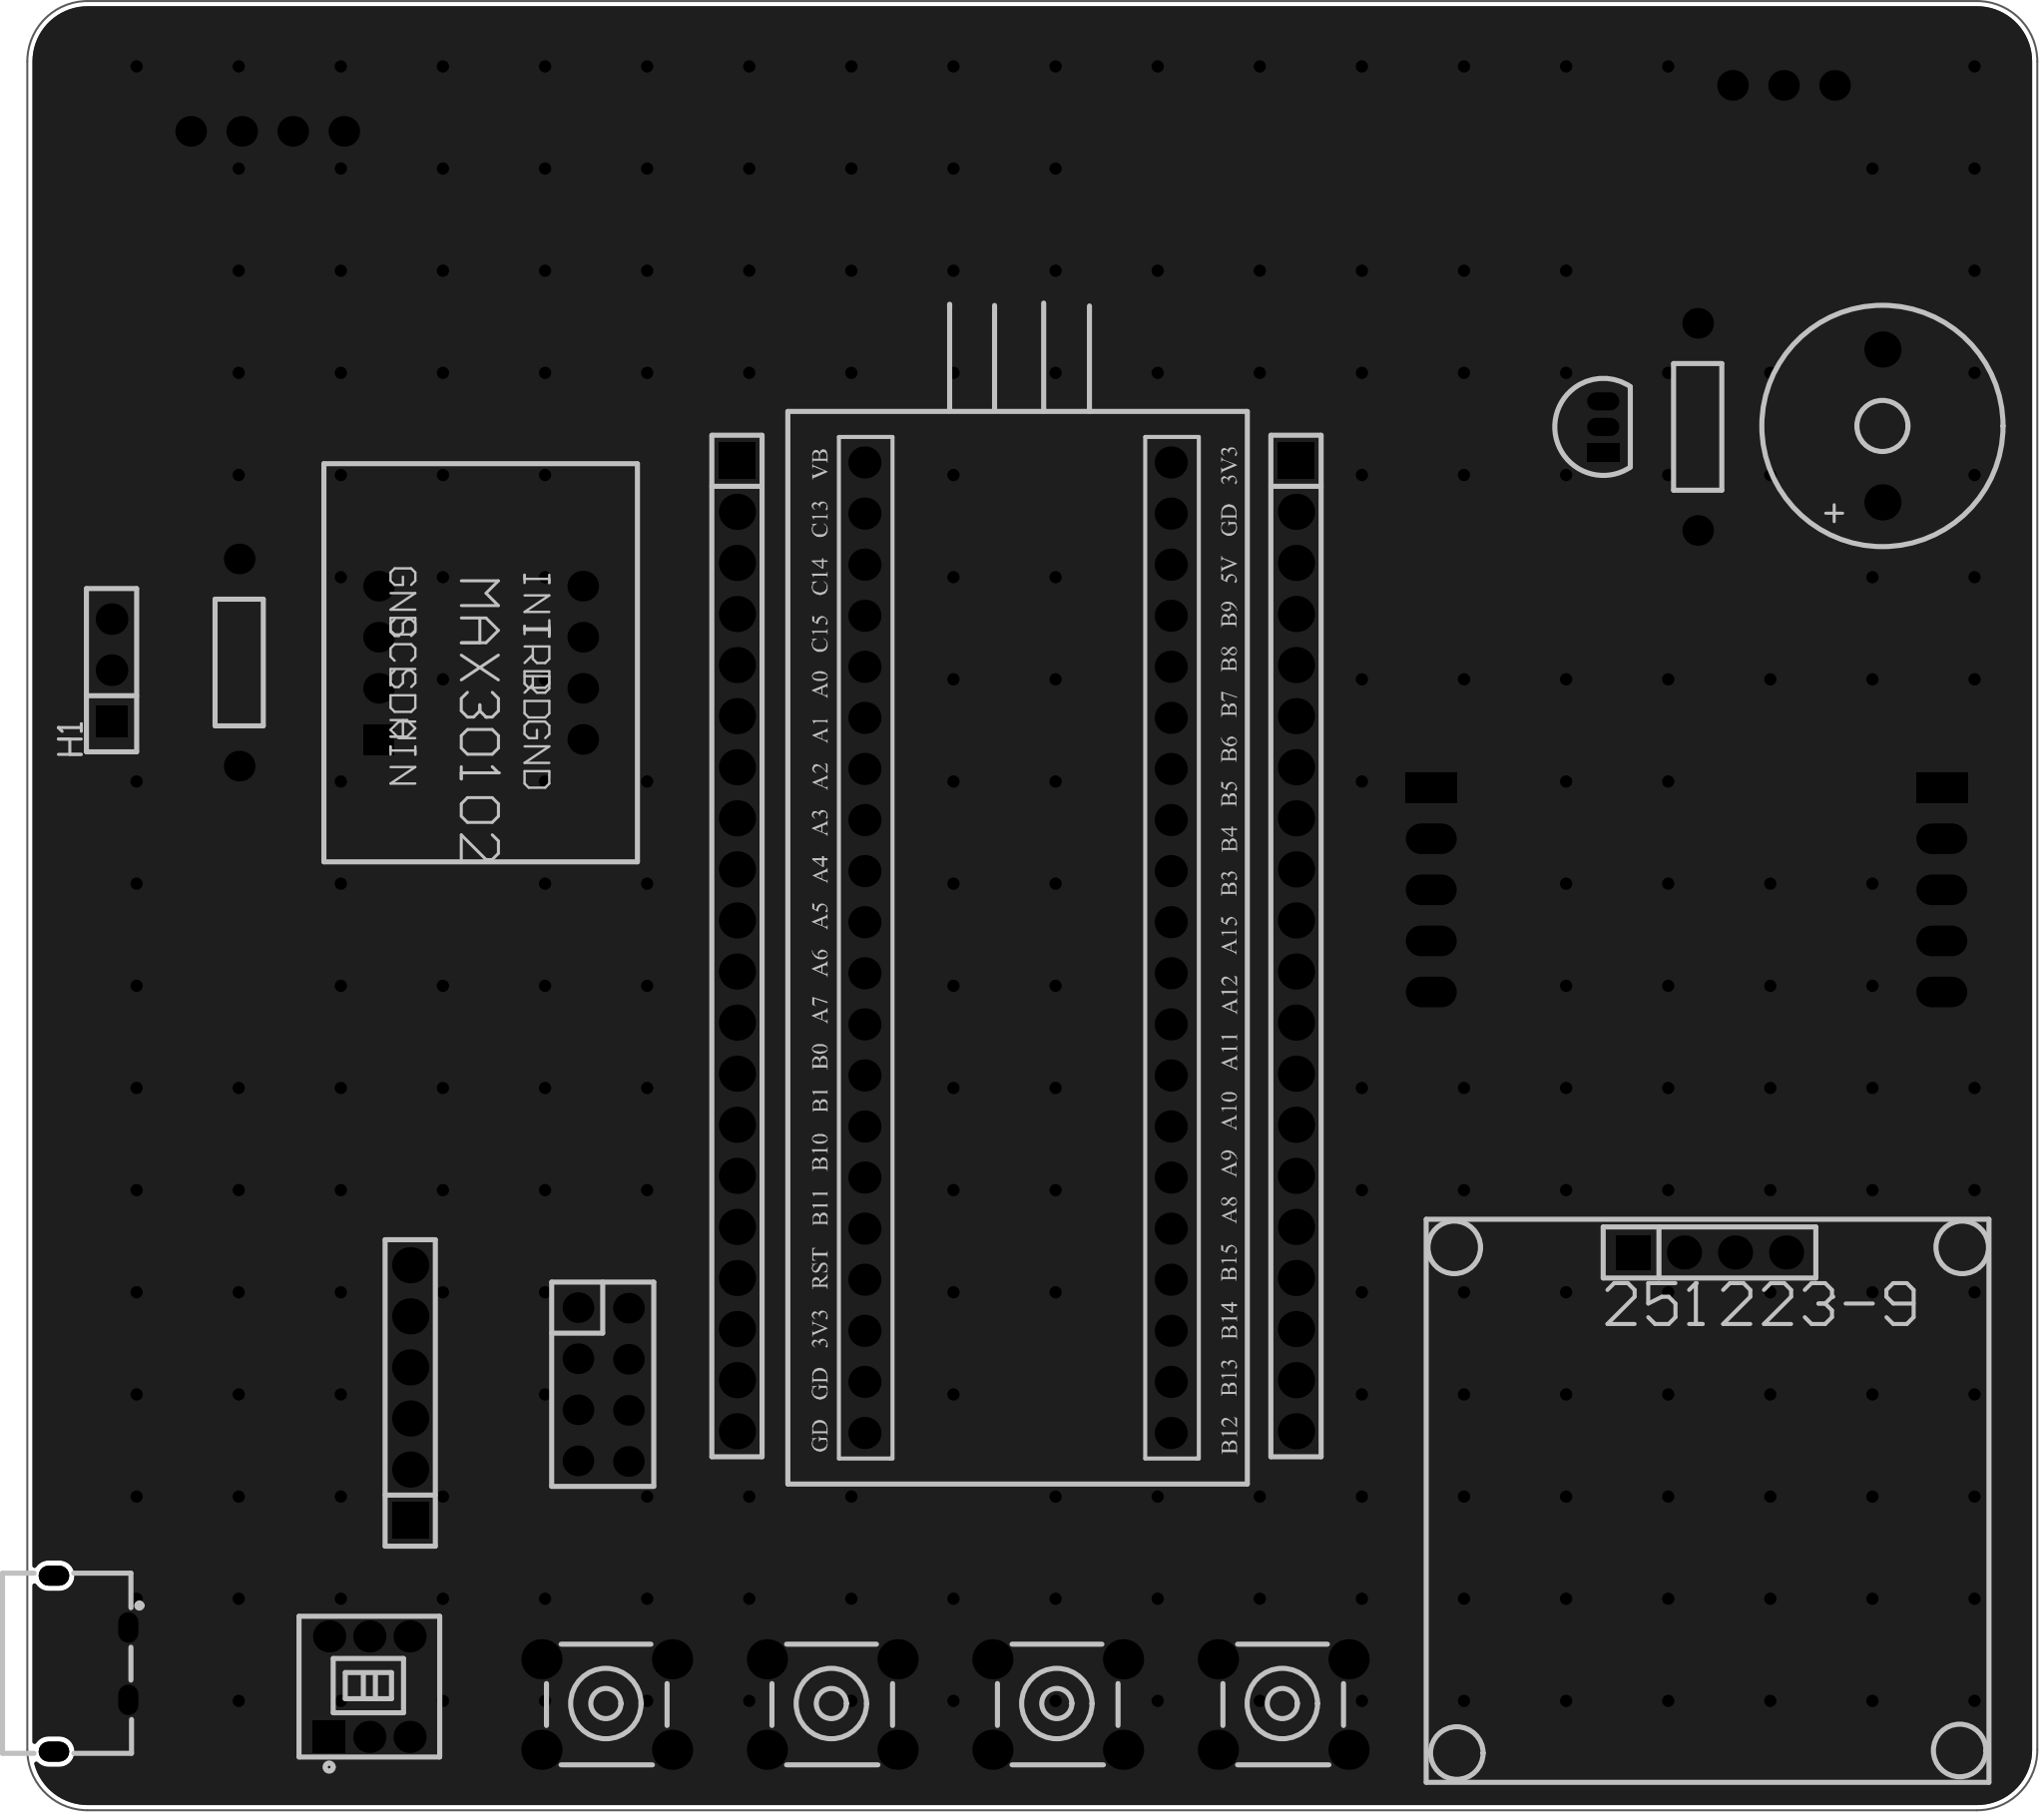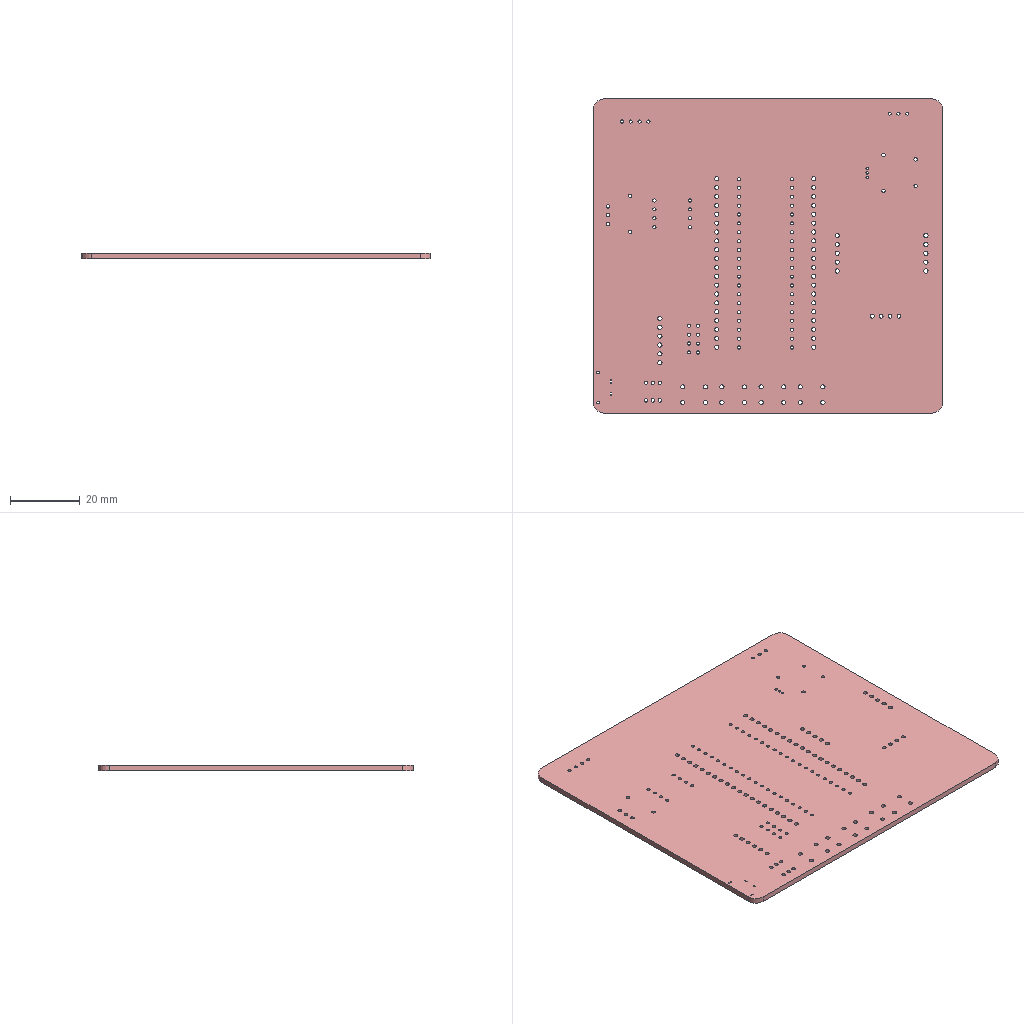Circuit board layout | Altium Designer | box 100 x 90 x 1.6 mm
Layer stack:
# Altium Designer layer stack of  (unit mm; dielectric type: 0 none, 1 core, 2 prepreg, 3 surface material)
index,name,kind,layer,copper_thickness_mm,dielectric_type,dielectric_thickness_mm,dielectric_material,dielectric_constant
0,Top Paste Mask Layer,other,,,,,,
1,Top Silkscreen Layer,other,,,,,,
2,Top Solder Mask Layer,dielectric,,,3,0.01,,3.3
3,Top Layer,copper,Top Layer,0.035,,,,
4,Dielectric1,dielectric,,,3,1.51,FR4,4.5
5,Bottom Layer,copper,Bottom Layer,0.035,,,,
6,Bottom Solder Mask Layer,dielectric,,,3,0.01,,3.3
7,Bottom Silkscreen Layer,other,,,,,,
8,Bottom Paste Mask Layer,other,,,,,,
# drill layer pairs: low layer,high layer
drill_pair,Top Layer,Bottom Layer
Part placement:
Designator,Comment,Layer,Footprint,Center-X(mm),Center-Y(mm),Rotation
H2,2.54-1*4P female,TopLayer,HDR-TH_4P-P2.54-V-F,165.672,135.255,0
H3,,TopLayer,HDR-TH_20P-P2.54-V-M-1,145.097,150.495,270
H4,,TopLayer,HDR-TH_20P-P2.54-V-M-1,117.284,150.495,270
H7,,TopLayer,HDR-TH_6P-P2.54-V-M-1,101.028,128.27,90
KEY1,Button 1,TopLayer,KEY-TH_4P-L6.0-W6.0-P4.50-LS7.5,110.808,112.776,0
KEY2,Button 5,TopLayer,KEY-TH_4P-L6.0-W6.0-P4.50-LS7.5,122.026,112.776,0
KEY3,Button 2,TopLayer,KEY-TH_4P-L6.0-W6.0-P4.50-LS7.5,133.244,112.776,0
KEY4,Button 4,TopLayer,KEY-TH_4P-L6.0-W6.0-P4.50-LS7.5,144.463,112.776,0
R98,4.7kΩ,TopLayer,Res_1/4W,92.519,164.592,90
U44,,TopLayer,STM32最小系统板,131.246,150.409,0
U89,,TopLayer,MAX30102,104.534,164.58,270
U98,,TopLayer,WiFi封装,110.629,128.688,90
SW8,TK-6700-1,TopLayer,SW-TH_TK-6700-1,98.996,113.665,0
U86,,TopLayer,ADXL345,164.529,153.289,0
USB2,KH-TYPE-C-2P,TopLayer,USB-SMD_KH-TYPE-C-2P,85.153,114.808,270
BUZZER3,2.3kHz,TopLayer,BUZ-TH_BD12.0-P7.60-D0.6-FD,174.274,176.356,90
Q17,,TopLayer,S8050_TO_92,160.384,176.31,90
R116,1kΩ,TopLayer,Res_1/4W,165.083,176.31,270
U1,,TopLayer,温湿度,169.355,193.294,180
U118,,TopLayer,MQ-X插件,93.916,191.008,90
H1,,TopLayer,HDR-TH_3P-P2.54-V-F,86.169,164.211,90
Pad and via stacks:
# Altium Designer via and pad stacks of  (unit mm). Each distinct definition once, with the count of objects using it.
# via: kind,start_layer,end_layer,hole_mm,diameter_mm,mode(0 simple;1 top-mid-bottom;2 full stack),diameter_per_layer,count,example_net
# pad: kind,layer,hole_mm,hole_type(0 round;1 square;2 slot),plating,top_size,top_shape(1 round;2 rect;3 octagon;9 rounded rect),mid_size,bottom_size,mode,footprint,size_per_layer,count,example
pad,Multi-Layer,1.1,0,plated,1.7x1.7,2,1.7x1.7,1.7x1.7,0,HDR-TH_4P-P2.54-V-F,,1,H2.1
pad,Multi-Layer,1.1,0,plated,1.7x1.7,1,1.7x1.7,1.7x1.7,0,HDR-TH_4P-P2.54-V-F,,3,H2.2
pad,Multi-Layer,1.2,0,plated,1.8x1.8,1,1.8x1.8,1.8x1.8,0,HDR-TH_20P-P2.54-V-M-1,,38,H3.20
pad,Multi-Layer,1.2,0,plated,1.8x1.8,2,1.8x1.8,1.8x1.8,0,HDR-TH_20P-P2.54-V-M-1,,2,H3.1
pad,Multi-Layer,1.2,0,plated,1.8x1.8,1,1.8x1.8,1.8x1.8,0,HDR-TH_6P-P2.54-V-M-1,,5,H7.6
pad,Multi-Layer,1.2,0,plated,1.8x1.8,2,1.8x1.8,1.8x1.8,0,HDR-TH_6P-P2.54-V-M-1,,1,H7.1
pad,Multi-Layer,1.2,0,plated,2x2,1,2x2,2x2,0,KEY-TH_4P-L6.0-W6.0-P4.50-LS7.5,,16,KEY1.1
pad,Multi-Layer,1,0,plated,1.524x1.524,1,1.524x1.524,1.524x1.524,0,Res_1/4W,,4,R98.1
pad,Multi-Layer,0.9,0,plated,1.6x1.6,1,1.6x1.6,1.6x1.6,0,STM32\u00D7\u00EE\u00D0\u00A1\u00CF\u00B5\u00CD\u00B3\u00B0\u00E5,,40,U44.40
pad,Multi-Layer,0.9144,0,plated,1.524x1.524,1,1.524x1.524,1.524x1.524,0,MAX30102,,7,U89.1
pad,Multi-Layer,0.9144,0,plated,1.524x1.524,2,1.524x1.524,1.524x1.524,0,MAX30102,,1,U89.8
pad,Multi-Layer,0.9144,0,plated,1.524x1.524,1,1.524x1.524,1.524x1.524,0,WiFi\u00B7\u00E2\u00D7\u00B0,,8,U98.1
pad,Multi-Layer,1,0,plated,1.6x1.6,2,1.6x1.6,1.6x1.6,0,SW-TH_TK-6700-1,,1,SW8.1
pad,Multi-Layer,1,0,plated,1.6x1.6,1,1.6x1.6,1.6x1.6,0,SW-TH_TK-6700-1,,5,SW8.2
pad,Multi-Layer,1.2,0,plated,1.524x2.54,1,1.524x2.54,1.524x2.54,0,ADXL345,,8,U86.5
pad,Multi-Layer,1.2,0,plated,1.524x2.54,2,1.524x2.54,1.524x2.54,0,ADXL345,,2,U86.1
pad,Multi-Layer,0.45,2,plated,1x1.524,1,1x1.524,1x1.524,0,USB-SMD_KH-TYPE-C-2P,,2,USB2.1
pad,Multi-Layer,0.5,2,plated,1x1.524,1,1x1.524,1x1.524,0,USB-SMD_KH-TYPE-C-2P,,2,USB2.3
pad,Multi-Layer,1,0,plated,1.8x1.8,1,1.8x1.8,1.8x1.8,0,BUZ-TH_BD12.0-P7.60-D0.6-FD,,2,BUZZER3.2
pad,Multi-Layer,0.701,0,plated,0.8992x1.6,2,0.8992x1.6,0.8992x1.6,0,S8050_TO_92,,1,Q17.1
pad,Multi-Layer,0.701,0,plated,0.8992x1.6,1,0.8992x1.6,0.8992x1.6,0,S8050_TO_92,,2,Q17.2
pad,Multi-Layer,0.9144,0,plated,1.524x1.524,1,1.524x1.524,1.524x1.524,0,\u00CE\u00C2\u00CA\u00AA\u00B6\u00C8,,3,U1.1
pad,Multi-Layer,0.9144,0,plated,1.524x1.524,1,1.524x1.524,1.524x1.524,0,MQ-X\u00B2\u00E5\u00BC\u00FE,,4,U118.1
pad,Multi-Layer,1.02,0,plated,1.575x1.575,1,1.575x1.575,1.575x1.575,0,HDR-TH_3P-P2.54-V-F,,2,H1.3
pad,Multi-Layer,1.02,0,plated,1.575x1.575,2,1.575x1.575,1.575x1.575,0,HDR-TH_3P-P2.54-V-F,,1,H1.1
via,Top Layer,Bottom Layer,0.3048,0.61,0,,229,GND
Copper pours:
name,layer,net,type(0 solid;1 hatched;2 none)
Bottom Layer-GND,Bottom Layer,GND,0
Top Layer-GND,Top Layer,GND,0